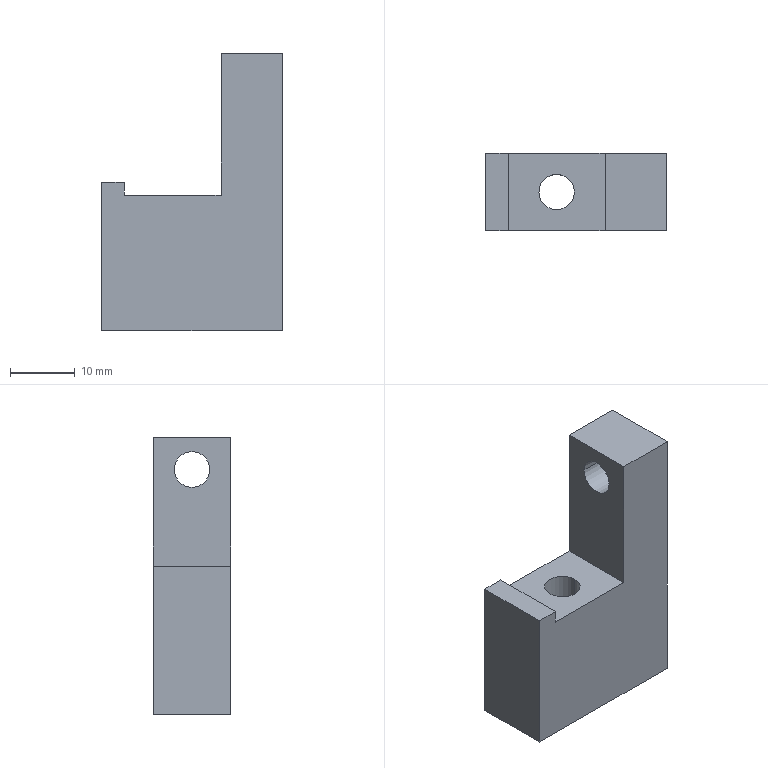Part | STEP file | 11-FG-E01411 | 1 solid | 17 faces | box 28 x 12 x 43 mm | volume 8595 mm3 | plane 11 | cylinder 6 | commonest cylinder face diameters 5.5 x4 10 x2
STEP:
#1=CARTESIAN_POINT('',(4.5,-2.75,38.));
#2=VERTEX_POINT('',#1);
#3=CARTESIAN_POINT('',(4.5,2.75,38.));
#4=VERTEX_POINT('',#3);
#5=CARTESIAN_POINT('',(4.5,0.,38.));
#6=DIRECTION('',(1.,0.,0.));
#7=DIRECTION('',(0.,0.,-1.));
#8=AXIS2_PLACEMENT_3D('',#5,#6,#7);
#9=CIRCLE('',#8,2.75);
#10=EDGE_CURVE('',#2,#4,#9,.T.);
#11=ORIENTED_EDGE('',*,*,#10,.F.);
#12=CARTESIAN_POINT('',(14.,-2.75,38.));
#13=VERTEX_POINT('',#12);
#14=CARTESIAN_POINT('',(4.,-2.75,38.));
#15=DIRECTION('',(1.,0.,0.));
#16=VECTOR('',#15,1000.);
#17=LINE('',#14,#16);
#18=EDGE_CURVE('',#2,#13,#17,.T.);
#19=ORIENTED_EDGE('',*,*,#18,.T.);
#20=CARTESIAN_POINT('',(14.,2.75,38.));
#21=VERTEX_POINT('',#20);
#22=CARTESIAN_POINT('',(14.,0.,38.));
#23=DIRECTION('',(1.,0.,0.));
#24=DIRECTION('',(0.,1.,0.));
#25=AXIS2_PLACEMENT_3D('',#22,#23,#24);
#26=CIRCLE('',#25,2.75);
#27=EDGE_CURVE('',#13,#21,#26,.T.);
#28=ORIENTED_EDGE('',*,*,#27,.T.);
#29=CARTESIAN_POINT('',(4.,2.75,38.));
#30=DIRECTION('',(1.,0.,0.));
#31=VECTOR('',#30,1000.);
#32=LINE('',#29,#31);
#33=EDGE_CURVE('',#4,#21,#32,.T.);
#34=ORIENTED_EDGE('',*,*,#33,.F.);
#35=EDGE_LOOP('',(#11,#19,#28,#34));
#36=FACE_OUTER_BOUND('',#35,.T.);
#37=CARTESIAN_POINT('',(4.,0.,38.));
#38=DIRECTION('',(1.,0.,0.));
#39=DIRECTION('',(0.,1.,0.));
#40=AXIS2_PLACEMENT_3D('',#37,#38,#39);
#41=CYLINDRICAL_SURFACE('',#40,2.75);
#42=ADVANCED_FACE('',(#36),#41,.F.);
#43=CARTESIAN_POINT('',(2.,0.,6.));
#44=VERTEX_POINT('',#43);
#45=CARTESIAN_POINT('',(-8.,0.,6.));
#46=VERTEX_POINT('',#45);
#47=CARTESIAN_POINT('',(-3.,0.,6.));
#48=DIRECTION('',(0.,0.,-1.));
#49=DIRECTION('',(-1.,0.,0.));
#50=AXIS2_PLACEMENT_3D('',#47,#48,#49);
#51=CIRCLE('',#50,5.);
#52=EDGE_CURVE('',#44,#46,#51,.T.);
#53=ORIENTED_EDGE('',*,*,#52,.F.);
#54=CARTESIAN_POINT('',(2.,0.,0.));
#55=VERTEX_POINT('',#54);
#56=CARTESIAN_POINT('',(2.,0.,6.));
#57=DIRECTION('',(0.,0.,-1.));
#58=VECTOR('',#57,1000.);
#59=LINE('',#56,#58);
#60=EDGE_CURVE('',#44,#55,#59,.T.);
#61=ORIENTED_EDGE('',*,*,#60,.T.);
#62=CARTESIAN_POINT('',(-8.,0.,0.));
#63=VERTEX_POINT('',#62);
#64=CARTESIAN_POINT('',(-3.,0.,0.));
#65=DIRECTION('',(0.,0.,-1.));
#66=DIRECTION('',(-1.,0.,0.));
#67=AXIS2_PLACEMENT_3D('',#64,#65,#66);
#68=CIRCLE('',#67,5.);
#69=EDGE_CURVE('',#55,#63,#68,.T.);
#70=ORIENTED_EDGE('',*,*,#69,.T.);
#71=CARTESIAN_POINT('',(-8.,0.,6.));
#72=DIRECTION('',(0.,0.,-1.));
#73=VECTOR('',#72,1000.);
#74=LINE('',#71,#73);
#75=EDGE_CURVE('',#46,#63,#74,.T.);
#76=ORIENTED_EDGE('',*,*,#75,.F.);
#77=EDGE_LOOP('',(#53,#61,#70,#76));
#78=FACE_OUTER_BOUND('',#77,.T.);
#79=CARTESIAN_POINT('',(-3.,0.,6.));
#80=DIRECTION('',(0.,0.,-1.));
#81=DIRECTION('',(-1.,0.,0.));
#82=AXIS2_PLACEMENT_3D('',#79,#80,#81);
#83=CYLINDRICAL_SURFACE('',#82,5.);
#84=ADVANCED_FACE('',(#78),#83,.F.);
#85=CARTESIAN_POINT('',(-5.75,0.,21.));
#86=VERTEX_POINT('',#85);
#87=CARTESIAN_POINT('',(-0.25,0.,21.));
#88=VERTEX_POINT('',#87);
#89=CARTESIAN_POINT('',(-3.,0.,21.));
#90=DIRECTION('',(0.,0.,1.));
#91=DIRECTION('',(-1.,0.,0.));
#92=AXIS2_PLACEMENT_3D('',#89,#90,#91);
#93=CIRCLE('',#92,2.75);
#94=EDGE_CURVE('',#86,#88,#93,.T.);
#95=ORIENTED_EDGE('',*,*,#94,.T.);
#96=CARTESIAN_POINT('',(-0.25,0.,6.));
#97=VERTEX_POINT('',#96);
#98=CARTESIAN_POINT('',(-0.25,0.,23.));
#99=DIRECTION('',(0.,0.,-1.));
#100=VECTOR('',#99,1000.);
#101=LINE('',#98,#100);
#102=EDGE_CURVE('',#88,#97,#101,.T.);
#103=ORIENTED_EDGE('',*,*,#102,.T.);
#104=CARTESIAN_POINT('',(-5.75,0.,6.));
#105=VERTEX_POINT('',#104);
#106=CARTESIAN_POINT('',(-3.,0.,6.));
#107=DIRECTION('',(0.,0.,1.));
#108=DIRECTION('',(-1.,0.,0.));
#109=AXIS2_PLACEMENT_3D('',#106,#107,#108);
#110=CIRCLE('',#109,2.75);
#111=EDGE_CURVE('',#105,#97,#110,.T.);
#112=ORIENTED_EDGE('',*,*,#111,.F.);
#113=CARTESIAN_POINT('',(-5.75,0.,23.));
#114=DIRECTION('',(0.,0.,-1.));
#115=VECTOR('',#114,1000.);
#116=LINE('',#113,#115);
#117=EDGE_CURVE('',#86,#105,#116,.T.);
#118=ORIENTED_EDGE('',*,*,#117,.F.);
#119=EDGE_LOOP('',(#95,#103,#112,#118));
#120=FACE_OUTER_BOUND('',#119,.T.);
#121=CARTESIAN_POINT('',(-3.,0.,23.));
#122=DIRECTION('',(0.,0.,-1.));
#123=DIRECTION('',(-1.,0.,0.));
#124=AXIS2_PLACEMENT_3D('',#121,#122,#123);
#125=CYLINDRICAL_SURFACE('',#124,2.75);
#126=ADVANCED_FACE('',(#120),#125,.F.);
#127=ORIENTED_EDGE('',*,*,#102,.F.);
#128=CARTESIAN_POINT('',(-3.,0.,21.));
#129=DIRECTION('',(0.,0.,1.));
#130=DIRECTION('',(-1.,0.,0.));
#131=AXIS2_PLACEMENT_3D('',#128,#129,#130);
#132=CIRCLE('',#131,2.75);
#133=EDGE_CURVE('',#88,#86,#132,.T.);
#134=ORIENTED_EDGE('',*,*,#133,.T.);
#135=ORIENTED_EDGE('',*,*,#117,.T.);
#136=CARTESIAN_POINT('',(-3.,0.,6.));
#137=DIRECTION('',(0.,0.,1.));
#138=DIRECTION('',(-1.,0.,0.));
#139=AXIS2_PLACEMENT_3D('',#136,#137,#138);
#140=CIRCLE('',#139,2.75);
#141=EDGE_CURVE('',#97,#105,#140,.T.);
#142=ORIENTED_EDGE('',*,*,#141,.F.);
#143=EDGE_LOOP('',(#127,#134,#135,#142));
#144=FACE_OUTER_BOUND('',#143,.T.);
#145=CARTESIAN_POINT('',(-3.,0.,23.));
#146=DIRECTION('',(0.,0.,-1.));
#147=DIRECTION('',(-1.,0.,0.));
#148=AXIS2_PLACEMENT_3D('',#145,#146,#147);
#149=CYLINDRICAL_SURFACE('',#148,2.75);
#150=ADVANCED_FACE('',(#144),#149,.F.);
#151=CARTESIAN_POINT('',(14.,0.,38.));
#152=DIRECTION('',(1.,0.,0.));
#153=DIRECTION('',(0.,1.,0.));
#154=AXIS2_PLACEMENT_3D('',#151,#152,#153);
#155=CIRCLE('',#154,2.75);
#156=EDGE_CURVE('',#21,#13,#155,.T.);
#157=ORIENTED_EDGE('',*,*,#156,.F.);
#158=ORIENTED_EDGE('',*,*,#27,.F.);
#159=EDGE_LOOP('',(#157,#158));
#160=FACE_BOUND('',#159,.T.);
#161=CARTESIAN_POINT('',(14.,-6.,0.));
#162=VERTEX_POINT('',#161);
#163=CARTESIAN_POINT('',(14.,6.,0.));
#164=VERTEX_POINT('',#163);
#165=CARTESIAN_POINT('',(14.,6.,0.));
#166=DIRECTION('',(0.,1.,0.));
#167=VECTOR('',#166,1000.);
#168=LINE('',#165,#167);
#169=EDGE_CURVE('',#162,#164,#168,.T.);
#170=ORIENTED_EDGE('',*,*,#169,.T.);
#171=CARTESIAN_POINT('',(14.,6.,43.));
#172=VERTEX_POINT('',#171);
#173=CARTESIAN_POINT('',(14.,6.,23.));
#174=DIRECTION('',(0.,0.,-1.));
#175=VECTOR('',#174,1000.);
#176=LINE('',#173,#175);
#177=EDGE_CURVE('',#172,#164,#176,.T.);
#178=ORIENTED_EDGE('',*,*,#177,.F.);
#179=CARTESIAN_POINT('',(14.,-6.,43.));
#180=VERTEX_POINT('',#179);
#181=CARTESIAN_POINT('',(14.,6.,43.));
#182=DIRECTION('',(0.,1.,0.));
#183=VECTOR('',#182,1000.);
#184=LINE('',#181,#183);
#185=EDGE_CURVE('',#180,#172,#184,.T.);
#186=ORIENTED_EDGE('',*,*,#185,.F.);
#187=CARTESIAN_POINT('',(14.,-6.,23.));
#188=DIRECTION('',(0.,0.,-1.));
#189=VECTOR('',#188,1000.);
#190=LINE('',#187,#189);
#191=EDGE_CURVE('',#180,#162,#190,.T.);
#192=ORIENTED_EDGE('',*,*,#191,.T.);
#193=EDGE_LOOP('',(#170,#178,#186,#192));
#194=FACE_OUTER_BOUND('',#193,.T.);
#195=CARTESIAN_POINT('',(14.,6.,23.));
#196=DIRECTION('',(-1.,0.,0.));
#197=DIRECTION('',(0.,-1.,0.));
#198=AXIS2_PLACEMENT_3D('',#195,#196,#197);
#199=PLANE('',#198);
#200=ADVANCED_FACE('',(#160,#194),#199,.F.);
#201=CARTESIAN_POINT('',(-10.5,6.,21.));
#202=VERTEX_POINT('',#201);
#203=CARTESIAN_POINT('',(4.5,6.,21.));
#204=VERTEX_POINT('',#203);
#205=CARTESIAN_POINT('',(-14.,6.,21.));
#206=DIRECTION('',(1.,0.,0.));
#207=VECTOR('',#206,1000.);
#208=LINE('',#205,#207);
#209=EDGE_CURVE('',#202,#204,#208,.T.);
#210=ORIENTED_EDGE('',*,*,#209,.T.);
#211=CARTESIAN_POINT('',(4.5,6.,43.));
#212=VERTEX_POINT('',#211);
#213=CARTESIAN_POINT('',(4.5,6.,23.));
#214=DIRECTION('',(0.,0.,1.));
#215=VECTOR('',#214,1000.);
#216=LINE('',#213,#215);
#217=EDGE_CURVE('',#204,#212,#216,.T.);
#218=ORIENTED_EDGE('',*,*,#217,.T.);
#219=CARTESIAN_POINT('',(14.,6.,43.));
#220=DIRECTION('',(-1.,0.,0.));
#221=VECTOR('',#220,1000.);
#222=LINE('',#219,#221);
#223=EDGE_CURVE('',#172,#212,#222,.T.);
#224=ORIENTED_EDGE('',*,*,#223,.F.);
#225=ORIENTED_EDGE('',*,*,#177,.T.);
#226=CARTESIAN_POINT('',(-14.,6.,0.));
#227=VERTEX_POINT('',#226);
#228=CARTESIAN_POINT('',(-14.,6.,0.));
#229=DIRECTION('',(-1.,0.,0.));
#230=VECTOR('',#229,1000.);
#231=LINE('',#228,#230);
#232=EDGE_CURVE('',#164,#227,#231,.T.);
#233=ORIENTED_EDGE('',*,*,#232,.T.);
#234=CARTESIAN_POINT('',(-14.,6.,23.));
#235=VERTEX_POINT('',#234);
#236=CARTESIAN_POINT('',(-14.,6.,23.));
#237=DIRECTION('',(0.,0.,-1.));
#238=VECTOR('',#237,1000.);
#239=LINE('',#236,#238);
#240=EDGE_CURVE('',#235,#227,#239,.T.);
#241=ORIENTED_EDGE('',*,*,#240,.F.);
#242=CARTESIAN_POINT('',(-10.5,6.,23.));
#243=VERTEX_POINT('',#242);
#244=CARTESIAN_POINT('',(-14.,6.,23.));
#245=DIRECTION('',(-1.,0.,0.));
#246=VECTOR('',#245,1000.);
#247=LINE('',#244,#246);
#248=EDGE_CURVE('',#243,#235,#247,.T.);
#249=ORIENTED_EDGE('',*,*,#248,.F.);
#250=CARTESIAN_POINT('',(-10.5,6.,23.));
#251=DIRECTION('',(0.,0.,-1.));
#252=VECTOR('',#251,1000.);
#253=LINE('',#250,#252);
#254=EDGE_CURVE('',#243,#202,#253,.T.);
#255=ORIENTED_EDGE('',*,*,#254,.T.);
#256=EDGE_LOOP('',(#210,#218,#224,#225,#233,#241,#249,#255));
#257=FACE_OUTER_BOUND('',#256,.T.);
#258=CARTESIAN_POINT('',(-14.,6.,23.));
#259=DIRECTION('',(0.,-1.,0.));
#260=DIRECTION('',(0.,0.,-1.));
#261=AXIS2_PLACEMENT_3D('',#258,#259,#260);
#262=PLANE('',#261);
#263=ADVANCED_FACE('',(#257),#262,.F.);
#264=CARTESIAN_POINT('',(-14.,-6.,0.));
#265=VERTEX_POINT('',#264);
#266=CARTESIAN_POINT('',(-14.,6.,0.));
#267=DIRECTION('',(0.,-1.,0.));
#268=VECTOR('',#267,1000.);
#269=LINE('',#266,#268);
#270=EDGE_CURVE('',#227,#265,#269,.T.);
#271=ORIENTED_EDGE('',*,*,#270,.T.);
#272=CARTESIAN_POINT('',(-14.,-6.,23.));
#273=VERTEX_POINT('',#272);
#274=CARTESIAN_POINT('',(-14.,-6.,23.));
#275=DIRECTION('',(0.,0.,-1.));
#276=VECTOR('',#275,1000.);
#277=LINE('',#274,#276);
#278=EDGE_CURVE('',#273,#265,#277,.T.);
#279=ORIENTED_EDGE('',*,*,#278,.F.);
#280=CARTESIAN_POINT('',(-14.,6.,23.));
#281=DIRECTION('',(0.,-1.,0.));
#282=VECTOR('',#281,1000.);
#283=LINE('',#280,#282);
#284=EDGE_CURVE('',#235,#273,#283,.T.);
#285=ORIENTED_EDGE('',*,*,#284,.F.);
#286=ORIENTED_EDGE('',*,*,#240,.T.);
#287=EDGE_LOOP('',(#271,#279,#285,#286));
#288=FACE_OUTER_BOUND('',#287,.T.);
#289=CARTESIAN_POINT('',(-14.,6.,23.));
#290=DIRECTION('',(1.,0.,0.));
#291=DIRECTION('',(0.,1.,0.));
#292=AXIS2_PLACEMENT_3D('',#289,#290,#291);
#293=PLANE('',#292);
#294=ADVANCED_FACE('',(#288),#293,.F.);
#295=ORIENTED_EDGE('',*,*,#191,.F.);
#296=CARTESIAN_POINT('',(4.5,-6.,43.));
#297=VERTEX_POINT('',#296);
#298=CARTESIAN_POINT('',(14.,-6.,43.));
#299=DIRECTION('',(1.,0.,0.));
#300=VECTOR('',#299,1000.);
#301=LINE('',#298,#300);
#302=EDGE_CURVE('',#297,#180,#301,.T.);
#303=ORIENTED_EDGE('',*,*,#302,.F.);
#304=CARTESIAN_POINT('',(4.5,-6.,21.));
#305=VERTEX_POINT('',#304);
#306=CARTESIAN_POINT('',(4.5,-6.,23.));
#307=DIRECTION('',(0.,0.,1.));
#308=VECTOR('',#307,1000.);
#309=LINE('',#306,#308);
#310=EDGE_CURVE('',#305,#297,#309,.T.);
#311=ORIENTED_EDGE('',*,*,#310,.F.);
#312=CARTESIAN_POINT('',(-10.5,-6.,21.));
#313=VERTEX_POINT('',#312);
#314=CARTESIAN_POINT('',(4.5,-6.,21.));
#315=DIRECTION('',(1.,0.,0.));
#316=VECTOR('',#315,1000.);
#317=LINE('',#314,#316);
#318=EDGE_CURVE('',#313,#305,#317,.T.);
#319=ORIENTED_EDGE('',*,*,#318,.F.);
#320=CARTESIAN_POINT('',(-10.5,-6.,23.));
#321=VERTEX_POINT('',#320);
#322=CARTESIAN_POINT('',(-10.5,-6.,23.));
#323=DIRECTION('',(0.,0.,-1.));
#324=VECTOR('',#323,1000.);
#325=LINE('',#322,#324);
#326=EDGE_CURVE('',#321,#313,#325,.T.);
#327=ORIENTED_EDGE('',*,*,#326,.F.);
#328=CARTESIAN_POINT('',(-14.,-6.,23.));
#329=DIRECTION('',(1.,0.,0.));
#330=VECTOR('',#329,1000.);
#331=LINE('',#328,#330);
#332=EDGE_CURVE('',#273,#321,#331,.T.);
#333=ORIENTED_EDGE('',*,*,#332,.F.);
#334=ORIENTED_EDGE('',*,*,#278,.T.);
#335=CARTESIAN_POINT('',(-14.,-6.,0.));
#336=DIRECTION('',(1.,0.,0.));
#337=VECTOR('',#336,1000.);
#338=LINE('',#335,#337);
#339=EDGE_CURVE('',#265,#162,#338,.T.);
#340=ORIENTED_EDGE('',*,*,#339,.T.);
#341=EDGE_LOOP('',(#295,#303,#311,#319,#327,#333,#334,#340));
#342=FACE_OUTER_BOUND('',#341,.T.);
#343=CARTESIAN_POINT('',(-14.,-6.,23.));
#344=DIRECTION('',(0.,1.,0.));
#345=DIRECTION('',(0.,0.,1.));
#346=AXIS2_PLACEMENT_3D('',#343,#344,#345);
#347=PLANE('',#346);
#348=ADVANCED_FACE('',(#342),#347,.F.);
#349=CARTESIAN_POINT('',(-10.5,-6.,23.));
#350=DIRECTION('',(0.,-1.,0.));
#351=VECTOR('',#350,1000.);
#352=LINE('',#349,#351);
#353=EDGE_CURVE('',#243,#321,#352,.T.);
#354=ORIENTED_EDGE('',*,*,#353,.F.);
#355=ORIENTED_EDGE('',*,*,#248,.T.);
#356=ORIENTED_EDGE('',*,*,#284,.T.);
#357=ORIENTED_EDGE('',*,*,#332,.T.);
#358=EDGE_LOOP('',(#354,#355,#356,#357));
#359=FACE_OUTER_BOUND('',#358,.T.);
#360=CARTESIAN_POINT('',(14.,-6.,23.));
#361=DIRECTION('',(0.,0.,1.));
#362=DIRECTION('',(1.,0.,0.));
#363=AXIS2_PLACEMENT_3D('',#360,#361,#362);
#364=PLANE('',#363);
#365=ADVANCED_FACE('',(#359),#364,.T.);
#366=CARTESIAN_POINT('',(-3.,0.,0.));
#367=DIRECTION('',(0.,0.,-1.));
#368=DIRECTION('',(-1.,0.,0.));
#369=AXIS2_PLACEMENT_3D('',#366,#367,#368);
#370=CIRCLE('',#369,5.);
#371=EDGE_CURVE('',#63,#55,#370,.T.);
#372=ORIENTED_EDGE('',*,*,#371,.F.);
#373=ORIENTED_EDGE('',*,*,#69,.F.);
#374=EDGE_LOOP('',(#372,#373));
#375=FACE_BOUND('',#374,.T.);
#376=ORIENTED_EDGE('',*,*,#169,.F.);
#377=ORIENTED_EDGE('',*,*,#339,.F.);
#378=ORIENTED_EDGE('',*,*,#270,.F.);
#379=ORIENTED_EDGE('',*,*,#232,.F.);
#380=EDGE_LOOP('',(#376,#377,#378,#379));
#381=FACE_OUTER_BOUND('',#380,.T.);
#382=CARTESIAN_POINT('',(14.,-6.,0.));
#383=DIRECTION('',(0.,0.,1.));
#384=DIRECTION('',(1.,0.,0.));
#385=AXIS2_PLACEMENT_3D('',#382,#383,#384);
#386=PLANE('',#385);
#387=ADVANCED_FACE('',(#375,#381),#386,.F.);
#388=CARTESIAN_POINT('',(-3.,0.,6.));
#389=DIRECTION('',(0.,0.,-1.));
#390=DIRECTION('',(-1.,0.,0.));
#391=AXIS2_PLACEMENT_3D('',#388,#389,#390);
#392=CIRCLE('',#391,5.);
#393=EDGE_CURVE('',#46,#44,#392,.T.);
#394=ORIENTED_EDGE('',*,*,#393,.T.);
#395=ORIENTED_EDGE('',*,*,#52,.T.);
#396=EDGE_LOOP('',(#394,#395));
#397=FACE_OUTER_BOUND('',#396,.T.);
#398=ORIENTED_EDGE('',*,*,#111,.T.);
#399=ORIENTED_EDGE('',*,*,#141,.T.);
#400=EDGE_LOOP('',(#398,#399));
#401=FACE_BOUND('',#400,.T.);
#402=CARTESIAN_POINT('',(-3.,0.,6.));
#403=DIRECTION('',(0.,0.,-1.));
#404=DIRECTION('',(-1.,0.,0.));
#405=AXIS2_PLACEMENT_3D('',#402,#403,#404);
#406=PLANE('',#405);
#407=ADVANCED_FACE('',(#397,#401),#406,.T.);
#408=ORIENTED_EDGE('',*,*,#60,.F.);
#409=ORIENTED_EDGE('',*,*,#393,.F.);
#410=ORIENTED_EDGE('',*,*,#75,.T.);
#411=ORIENTED_EDGE('',*,*,#371,.T.);
#412=EDGE_LOOP('',(#408,#409,#410,#411));
#413=FACE_OUTER_BOUND('',#412,.T.);
#414=CARTESIAN_POINT('',(-3.,0.,6.));
#415=DIRECTION('',(0.,0.,-1.));
#416=DIRECTION('',(-1.,0.,0.));
#417=AXIS2_PLACEMENT_3D('',#414,#415,#416);
#418=CYLINDRICAL_SURFACE('',#417,5.);
#419=ADVANCED_FACE('',(#413),#418,.F.);
#420=CARTESIAN_POINT('',(-10.5,9.,21.));
#421=DIRECTION('',(0.,-1.,0.));
#422=VECTOR('',#421,1000.);
#423=LINE('',#420,#422);
#424=EDGE_CURVE('',#202,#313,#423,.T.);
#425=ORIENTED_EDGE('',*,*,#424,.T.);
#426=ORIENTED_EDGE('',*,*,#318,.T.);
#427=CARTESIAN_POINT('',(4.5,9.,21.));
#428=DIRECTION('',(0.,-1.,0.));
#429=VECTOR('',#428,1000.);
#430=LINE('',#427,#429);
#431=EDGE_CURVE('',#204,#305,#430,.T.);
#432=ORIENTED_EDGE('',*,*,#431,.F.);
#433=ORIENTED_EDGE('',*,*,#209,.F.);
#434=EDGE_LOOP('',(#425,#426,#432,#433));
#435=FACE_OUTER_BOUND('',#434,.T.);
#436=ORIENTED_EDGE('',*,*,#94,.F.);
#437=ORIENTED_EDGE('',*,*,#133,.F.);
#438=EDGE_LOOP('',(#436,#437));
#439=FACE_BOUND('',#438,.T.);
#440=CARTESIAN_POINT('',(4.5,9.,21.));
#441=DIRECTION('',(0.,0.,-1.));
#442=DIRECTION('',(-1.,0.,0.));
#443=AXIS2_PLACEMENT_3D('',#440,#441,#442);
#444=PLANE('',#443);
#445=ADVANCED_FACE('',(#435,#439),#444,.F.);
#446=CARTESIAN_POINT('',(4.5,0.,38.));
#447=DIRECTION('',(1.,0.,0.));
#448=DIRECTION('',(0.,0.,-1.));
#449=AXIS2_PLACEMENT_3D('',#446,#447,#448);
#450=CIRCLE('',#449,2.75);
#451=EDGE_CURVE('',#4,#2,#450,.T.);
#452=ORIENTED_EDGE('',*,*,#451,.T.);
#453=ORIENTED_EDGE('',*,*,#10,.T.);
#454=EDGE_LOOP('',(#452,#453));
#455=FACE_BOUND('',#454,.T.);
#456=ORIENTED_EDGE('',*,*,#431,.T.);
#457=ORIENTED_EDGE('',*,*,#310,.T.);
#458=CARTESIAN_POINT('',(4.5,6.,43.));
#459=DIRECTION('',(0.,-1.,0.));
#460=VECTOR('',#459,1000.);
#461=LINE('',#458,#460);
#462=EDGE_CURVE('',#212,#297,#461,.T.);
#463=ORIENTED_EDGE('',*,*,#462,.F.);
#464=ORIENTED_EDGE('',*,*,#217,.F.);
#465=EDGE_LOOP('',(#456,#457,#463,#464));
#466=FACE_OUTER_BOUND('',#465,.T.);
#467=CARTESIAN_POINT('',(4.5,9.,23.));
#468=DIRECTION('',(1.,0.,0.));
#469=DIRECTION('',(0.,0.,-1.));
#470=AXIS2_PLACEMENT_3D('',#467,#468,#469);
#471=PLANE('',#470);
#472=ADVANCED_FACE('',(#455,#466),#471,.F.);
#473=ORIENTED_EDGE('',*,*,#353,.T.);
#474=ORIENTED_EDGE('',*,*,#326,.T.);
#475=ORIENTED_EDGE('',*,*,#424,.F.);
#476=ORIENTED_EDGE('',*,*,#254,.F.);
#477=EDGE_LOOP('',(#473,#474,#475,#476));
#478=FACE_OUTER_BOUND('',#477,.T.);
#479=CARTESIAN_POINT('',(-10.5,9.,23.));
#480=DIRECTION('',(-1.,0.,0.));
#481=DIRECTION('',(0.,0.,1.));
#482=AXIS2_PLACEMENT_3D('',#479,#480,#481);
#483=PLANE('',#482);
#484=ADVANCED_FACE('',(#478),#483,.F.);
#485=ORIENTED_EDGE('',*,*,#185,.T.);
#486=ORIENTED_EDGE('',*,*,#223,.T.);
#487=ORIENTED_EDGE('',*,*,#462,.T.);
#488=ORIENTED_EDGE('',*,*,#302,.T.);
#489=EDGE_LOOP('',(#485,#486,#487,#488));
#490=FACE_OUTER_BOUND('',#489,.T.);
#491=CARTESIAN_POINT('',(0.,0.,43.));
#492=DIRECTION('',(0.,0.,-1.));
#493=DIRECTION('',(-1.,0.,0.));
#494=AXIS2_PLACEMENT_3D('',#491,#492,#493);
#495=PLANE('',#494);
#496=ADVANCED_FACE('',(#490),#495,.F.);
#497=ORIENTED_EDGE('',*,*,#18,.F.);
#498=ORIENTED_EDGE('',*,*,#451,.F.);
#499=ORIENTED_EDGE('',*,*,#33,.T.);
#500=ORIENTED_EDGE('',*,*,#156,.T.);
#501=EDGE_LOOP('',(#497,#498,#499,#500));
#502=FACE_OUTER_BOUND('',#501,.T.);
#503=CARTESIAN_POINT('',(4.,0.,38.));
#504=DIRECTION('',(1.,0.,0.));
#505=DIRECTION('',(0.,1.,0.));
#506=AXIS2_PLACEMENT_3D('',#503,#504,#505);
#507=CYLINDRICAL_SURFACE('',#506,2.75);
#508=ADVANCED_FACE('',(#502),#507,.F.);
#509=CLOSED_SHELL('',(#42,#84,#126,#150,#200,#263,#294,#348,#365,#387,#407,#419,#445,#472,#484,#496,#508));
#510=MANIFOLD_SOLID_BREP('',#509);
#511=CARTESIAN_POINT('',(0.,0.,0.));
#512=DIRECTION('',(0.,0.,1.));
#513=DIRECTION('',(1.,0.,0.));
#514=AXIS2_PLACEMENT_3D('',#511,#512,#513);
#515=(LENGTH_UNIT()NAMED_UNIT(*)SI_UNIT(.MILLI.,.METRE.));
#516=UNCERTAINTY_MEASURE_WITH_UNIT(LENGTH_MEASURE(0.00001),#515,'','');
#517=(NAMED_UNIT(*)PLANE_ANGLE_UNIT()SI_UNIT($,.RADIAN.));
#518=(NAMED_UNIT(*)SI_UNIT($,.STERADIAN.)SOLID_ANGLE_UNIT());
#519=(GEOMETRIC_REPRESENTATION_CONTEXT(3)GLOBAL_UNCERTAINTY_ASSIGNED_CONTEXT((#516))GLOBAL_UNIT_ASSIGNED_CONTEXT((#515,#517,#518))REPRESENTATION_CONTEXT('',''));
#520=ADVANCED_BREP_SHAPE_REPRESENTATION('',(#510,#514),#519);